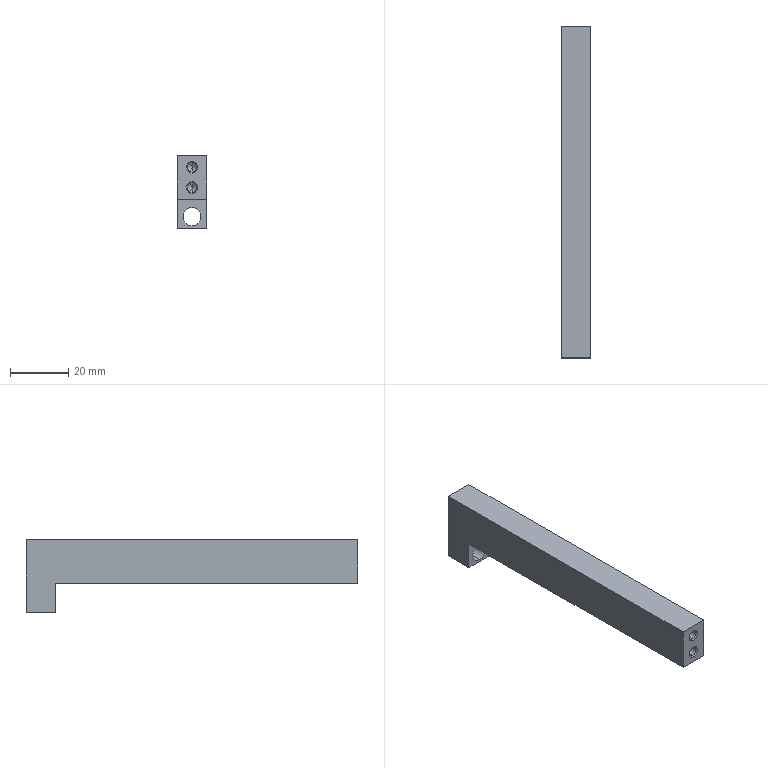Part | SolidWorks | features Extrusion 1, HoleWzd 1, ICE 1 | 1 solid | 22 faces | box 10 x 114 x 25 mm | volume 17594 mm3 | cone 8 | plane 8 | cylinder 6 | commonest cylinder face diameters 3.3 x4 6.2 x2
STEP:
#1=CARTESIAN_POINT('',(0.,0.375,-1.85));
#2=VERTEX_POINT('',#1);
#3=CARTESIAN_POINT('',(0.,0.375,-5.15));
#4=VERTEX_POINT('',#3);
#5=CARTESIAN_POINT('',(0.,0.375,-3.5));
#6=DIRECTION('',(0.,-1.,0.));
#7=DIRECTION('',(0.,0.,-1.));
#8=AXIS2_PLACEMENT_3D('',#5,#6,#7);
#9=CIRCLE('',#8,1.65);
#10=EDGE_CURVE('',#2,#4,#9,.T.);
#11=ORIENTED_EDGE('',*,*,#10,.F.);
#12=CARTESIAN_POINT('',(0.,0.,-1.475));
#13=VERTEX_POINT('',#12);
#14=CARTESIAN_POINT('',(0.,0.,-1.475));
#15=DIRECTION('',(0.,-0.7071,0.7071));
#16=VECTOR('',#15,1000.);
#17=LINE('',#14,#16);
#18=EDGE_CURVE('',#2,#13,#17,.T.);
#19=ORIENTED_EDGE('',*,*,#18,.T.);
#20=CARTESIAN_POINT('',(0.,0.,-5.525));
#21=VERTEX_POINT('',#20);
#22=CARTESIAN_POINT('',(0.,0.,-3.5));
#23=DIRECTION('',(0.,-1.,0.));
#24=DIRECTION('',(0.,0.,-1.));
#25=AXIS2_PLACEMENT_3D('',#22,#23,#24);
#26=CIRCLE('',#25,2.025);
#27=EDGE_CURVE('',#13,#21,#26,.T.);
#28=ORIENTED_EDGE('',*,*,#27,.T.);
#29=CARTESIAN_POINT('',(0.,0.,-5.525));
#30=DIRECTION('',(0.,-0.7071,-0.7071));
#31=VECTOR('',#30,1000.);
#32=LINE('',#29,#31);
#33=EDGE_CURVE('',#4,#21,#32,.T.);
#34=ORIENTED_EDGE('',*,*,#33,.F.);
#35=EDGE_LOOP('',(#11,#19,#28,#34));
#36=FACE_OUTER_BOUND('',#35,.T.);
#37=CARTESIAN_POINT('',(0.,0.,-3.5));
#38=DIRECTION('',(0.,-1.,0.));
#39=DIRECTION('',(0.,0.,-1.));
#40=AXIS2_PLACEMENT_3D('',#37,#38,#39);
#41=CONICAL_SURFACE('',#40,2.025,0.7854);
#42=ADVANCED_FACE('',(#36),#41,.F.);
#43=CARTESIAN_POINT('',(0.,11.5,-1.85));
#44=VERTEX_POINT('',#43);
#45=CARTESIAN_POINT('',(0.,11.5,-5.15));
#46=VERTEX_POINT('',#45);
#47=CARTESIAN_POINT('',(0.,11.5,-3.5));
#48=DIRECTION('',(0.,-1.,0.));
#49=DIRECTION('',(0.,0.,-1.));
#50=AXIS2_PLACEMENT_3D('',#47,#48,#49);
#51=CIRCLE('',#50,1.65);
#52=EDGE_CURVE('',#44,#46,#51,.T.);
#53=ORIENTED_EDGE('',*,*,#52,.F.);
#54=CARTESIAN_POINT('',(0.,0.,-1.85));
#55=DIRECTION('',(0.,-1.,0.));
#56=VECTOR('',#55,1000.);
#57=LINE('',#54,#56);
#58=EDGE_CURVE('',#44,#2,#57,.T.);
#59=ORIENTED_EDGE('',*,*,#58,.T.);
#60=ORIENTED_EDGE('',*,*,#10,.T.);
#61=CARTESIAN_POINT('',(0.,0.,-5.15));
#62=DIRECTION('',(0.,-1.,0.));
#63=VECTOR('',#62,1000.);
#64=LINE('',#61,#63);
#65=EDGE_CURVE('',#46,#4,#64,.T.);
#66=ORIENTED_EDGE('',*,*,#65,.F.);
#67=EDGE_LOOP('',(#53,#59,#60,#66));
#68=FACE_OUTER_BOUND('',#67,.T.);
#69=CARTESIAN_POINT('',(0.,0.,-3.5));
#70=DIRECTION('',(0.,-1.,0.));
#71=DIRECTION('',(0.,0.,-1.));
#72=AXIS2_PLACEMENT_3D('',#69,#70,#71);
#73=CYLINDRICAL_SURFACE('',#72,1.65);
#74=ADVANCED_FACE('',(#68),#73,.F.);
#75=CARTESIAN_POINT('',(0.,12.491,-3.5));
#76=VERTEX_POINT('',#75);
#77=CARTESIAN_POINT('',(0.,11.5,-5.15));
#78=DIRECTION('',(0.,-0.515,-0.8572));
#79=VECTOR('',#78,1000.);
#80=LINE('',#77,#79);
#81=EDGE_CURVE('',#76,#46,#80,.T.);
#82=ORIENTED_EDGE('',*,*,#81,.F.);
#83=CARTESIAN_POINT('',(0.,11.5,-1.85));
#84=DIRECTION('',(0.,-0.515,0.8572));
#85=VECTOR('',#84,1000.);
#86=LINE('',#83,#85);
#87=EDGE_CURVE('',#76,#44,#86,.T.);
#88=ORIENTED_EDGE('',*,*,#87,.T.);
#89=ORIENTED_EDGE('',*,*,#52,.T.);
#90=EDGE_LOOP('',(#82,#88,#89));
#91=FACE_OUTER_BOUND('',#90,.T.);
#92=CARTESIAN_POINT('',(0.,11.5,-3.5));
#93=DIRECTION('',(0.,-1.,0.));
#94=DIRECTION('',(0.,0.,-1.));
#95=AXIS2_PLACEMENT_3D('',#92,#93,#94);
#96=CONICAL_SURFACE('',#95,1.65,1.03);
#97=ADVANCED_FACE('',(#91),#96,.F.);
#98=CARTESIAN_POINT('',(0.,0.375,5.15));
#99=VERTEX_POINT('',#98);
#100=CARTESIAN_POINT('',(0.,0.375,1.85));
#101=VERTEX_POINT('',#100);
#102=CARTESIAN_POINT('',(0.,0.375,3.5));
#103=DIRECTION('',(0.,-1.,0.));
#104=DIRECTION('',(0.,0.,-1.));
#105=AXIS2_PLACEMENT_3D('',#102,#103,#104);
#106=CIRCLE('',#105,1.65);
#107=EDGE_CURVE('',#99,#101,#106,.T.);
#108=ORIENTED_EDGE('',*,*,#107,.F.);
#109=CARTESIAN_POINT('',(0.,0.,5.525));
#110=VERTEX_POINT('',#109);
#111=CARTESIAN_POINT('',(0.,0.,5.525));
#112=DIRECTION('',(0.,-0.7071,0.7071));
#113=VECTOR('',#112,1000.);
#114=LINE('',#111,#113);
#115=EDGE_CURVE('',#99,#110,#114,.T.);
#116=ORIENTED_EDGE('',*,*,#115,.T.);
#117=CARTESIAN_POINT('',(0.,0.,1.475));
#118=VERTEX_POINT('',#117);
#119=CARTESIAN_POINT('',(0.,0.,3.5));
#120=DIRECTION('',(0.,-1.,0.));
#121=DIRECTION('',(0.,0.,-1.));
#122=AXIS2_PLACEMENT_3D('',#119,#120,#121);
#123=CIRCLE('',#122,2.025);
#124=EDGE_CURVE('',#110,#118,#123,.T.);
#125=ORIENTED_EDGE('',*,*,#124,.T.);
#126=CARTESIAN_POINT('',(0.,0.,1.475));
#127=DIRECTION('',(0.,-0.7071,-0.7071));
#128=VECTOR('',#127,1000.);
#129=LINE('',#126,#128);
#130=EDGE_CURVE('',#101,#118,#129,.T.);
#131=ORIENTED_EDGE('',*,*,#130,.F.);
#132=EDGE_LOOP('',(#108,#116,#125,#131));
#133=FACE_OUTER_BOUND('',#132,.T.);
#134=CARTESIAN_POINT('',(0.,0.,3.5));
#135=DIRECTION('',(0.,-1.,0.));
#136=DIRECTION('',(0.,0.,-1.));
#137=AXIS2_PLACEMENT_3D('',#134,#135,#136);
#138=CONICAL_SURFACE('',#137,2.025,0.7854);
#139=ADVANCED_FACE('',(#133),#138,.F.);
#140=CARTESIAN_POINT('',(0.,11.5,5.15));
#141=VERTEX_POINT('',#140);
#142=CARTESIAN_POINT('',(0.,11.5,1.85));
#143=VERTEX_POINT('',#142);
#144=CARTESIAN_POINT('',(0.,11.5,3.5));
#145=DIRECTION('',(0.,-1.,0.));
#146=DIRECTION('',(0.,0.,-1.));
#147=AXIS2_PLACEMENT_3D('',#144,#145,#146);
#148=CIRCLE('',#147,1.65);
#149=EDGE_CURVE('',#141,#143,#148,.T.);
#150=ORIENTED_EDGE('',*,*,#149,.F.);
#151=CARTESIAN_POINT('',(0.,0.,5.15));
#152=DIRECTION('',(0.,-1.,0.));
#153=VECTOR('',#152,1000.);
#154=LINE('',#151,#153);
#155=EDGE_CURVE('',#141,#99,#154,.T.);
#156=ORIENTED_EDGE('',*,*,#155,.T.);
#157=ORIENTED_EDGE('',*,*,#107,.T.);
#158=CARTESIAN_POINT('',(0.,0.,1.85));
#159=DIRECTION('',(0.,-1.,0.));
#160=VECTOR('',#159,1000.);
#161=LINE('',#158,#160);
#162=EDGE_CURVE('',#143,#101,#161,.T.);
#163=ORIENTED_EDGE('',*,*,#162,.F.);
#164=EDGE_LOOP('',(#150,#156,#157,#163));
#165=FACE_OUTER_BOUND('',#164,.T.);
#166=CARTESIAN_POINT('',(0.,0.,3.5));
#167=DIRECTION('',(0.,-1.,0.));
#168=DIRECTION('',(0.,0.,-1.));
#169=AXIS2_PLACEMENT_3D('',#166,#167,#168);
#170=CYLINDRICAL_SURFACE('',#169,1.65);
#171=ADVANCED_FACE('',(#165),#170,.F.);
#172=CARTESIAN_POINT('',(0.,12.491,3.5));
#173=VERTEX_POINT('',#172);
#174=CARTESIAN_POINT('',(0.,11.5,1.85));
#175=DIRECTION('',(0.,-0.515,-0.8572));
#176=VECTOR('',#175,1000.);
#177=LINE('',#174,#176);
#178=EDGE_CURVE('',#173,#143,#177,.T.);
#179=ORIENTED_EDGE('',*,*,#178,.F.);
#180=CARTESIAN_POINT('',(0.,11.5,5.15));
#181=DIRECTION('',(0.,-0.515,0.8572));
#182=VECTOR('',#181,1000.);
#183=LINE('',#180,#182);
#184=EDGE_CURVE('',#173,#141,#183,.T.);
#185=ORIENTED_EDGE('',*,*,#184,.T.);
#186=ORIENTED_EDGE('',*,*,#149,.T.);
#187=EDGE_LOOP('',(#179,#185,#186));
#188=FACE_OUTER_BOUND('',#187,.T.);
#189=CARTESIAN_POINT('',(0.,11.5,3.5));
#190=DIRECTION('',(0.,-1.,0.));
#191=DIRECTION('',(0.,0.,-1.));
#192=AXIS2_PLACEMENT_3D('',#189,#190,#191);
#193=CONICAL_SURFACE('',#192,1.65,1.03);
#194=ADVANCED_FACE('',(#188),#193,.F.);
#195=CARTESIAN_POINT('',(0.,104.,-16.6));
#196=VERTEX_POINT('',#195);
#197=CARTESIAN_POINT('',(0.,104.,-10.4));
#198=VERTEX_POINT('',#197);
#199=CARTESIAN_POINT('',(0.,104.,-13.5));
#200=DIRECTION('',(0.,1.,0.));
#201=DIRECTION('',(0.,0.,1.));
#202=AXIS2_PLACEMENT_3D('',#199,#200,#201);
#203=CIRCLE('',#202,3.1);
#204=EDGE_CURVE('',#196,#198,#203,.T.);
#205=ORIENTED_EDGE('',*,*,#204,.F.);
#206=CARTESIAN_POINT('',(0.,114.,-16.6));
#207=VERTEX_POINT('',#206);
#208=CARTESIAN_POINT('',(0.,104.,-16.6));
#209=DIRECTION('',(0.,1.,0.));
#210=VECTOR('',#209,1000.);
#211=LINE('',#208,#210);
#212=EDGE_CURVE('',#196,#207,#211,.T.);
#213=ORIENTED_EDGE('',*,*,#212,.T.);
#214=CARTESIAN_POINT('',(0.,114.,-10.4));
#215=VERTEX_POINT('',#214);
#216=CARTESIAN_POINT('',(0.,114.,-13.5));
#217=DIRECTION('',(0.,1.,0.));
#218=DIRECTION('',(0.,0.,1.));
#219=AXIS2_PLACEMENT_3D('',#216,#217,#218);
#220=CIRCLE('',#219,3.1);
#221=EDGE_CURVE('',#207,#215,#220,.T.);
#222=ORIENTED_EDGE('',*,*,#221,.T.);
#223=CARTESIAN_POINT('',(0.,104.,-10.4));
#224=DIRECTION('',(0.,1.,0.));
#225=VECTOR('',#224,1000.);
#226=LINE('',#223,#225);
#227=EDGE_CURVE('',#198,#215,#226,.T.);
#228=ORIENTED_EDGE('',*,*,#227,.F.);
#229=EDGE_LOOP('',(#205,#213,#222,#228));
#230=FACE_OUTER_BOUND('',#229,.T.);
#231=CARTESIAN_POINT('',(0.,104.,-13.5));
#232=DIRECTION('',(0.,1.,0.));
#233=DIRECTION('',(0.,0.,1.));
#234=AXIS2_PLACEMENT_3D('',#231,#232,#233);
#235=CYLINDRICAL_SURFACE('',#234,3.1);
#236=ADVANCED_FACE('',(#230),#235,.F.);
#237=CARTESIAN_POINT('',(5.,0.,7.5));
#238=VERTEX_POINT('',#237);
#239=CARTESIAN_POINT('',(5.,0.,-7.5));
#240=VERTEX_POINT('',#239);
#241=CARTESIAN_POINT('',(5.,0.,7.5));
#242=DIRECTION('',(0.,0.,-1.));
#243=VECTOR('',#242,1000.);
#244=LINE('',#241,#243);
#245=EDGE_CURVE('',#238,#240,#244,.T.);
#246=ORIENTED_EDGE('',*,*,#245,.T.);
#247=CARTESIAN_POINT('',(5.,104.,-7.5));
#248=VERTEX_POINT('',#247);
#249=CARTESIAN_POINT('',(5.,114.,-7.5));
#250=DIRECTION('',(0.,-1.,0.));
#251=VECTOR('',#250,1000.);
#252=LINE('',#249,#251);
#253=EDGE_CURVE('',#248,#240,#252,.T.);
#254=ORIENTED_EDGE('',*,*,#253,.F.);
#255=CARTESIAN_POINT('',(5.,104.,-17.5));
#256=VERTEX_POINT('',#255);
#257=CARTESIAN_POINT('',(5.,104.,-7.5));
#258=DIRECTION('',(0.,0.,-1.));
#259=VECTOR('',#258,1000.);
#260=LINE('',#257,#259);
#261=EDGE_CURVE('',#248,#256,#260,.T.);
#262=ORIENTED_EDGE('',*,*,#261,.T.);
#263=CARTESIAN_POINT('',(5.,114.,-17.5));
#264=VERTEX_POINT('',#263);
#265=CARTESIAN_POINT('',(5.,104.,-17.5));
#266=DIRECTION('',(0.,1.,0.));
#267=VECTOR('',#266,1000.);
#268=LINE('',#265,#267);
#269=EDGE_CURVE('',#256,#264,#268,.T.);
#270=ORIENTED_EDGE('',*,*,#269,.T.);
#271=CARTESIAN_POINT('',(5.,114.,7.5));
#272=VERTEX_POINT('',#271);
#273=CARTESIAN_POINT('',(5.,114.,7.5));
#274=DIRECTION('',(0.,0.,-1.));
#275=VECTOR('',#274,1000.);
#276=LINE('',#273,#275);
#277=EDGE_CURVE('',#272,#264,#276,.T.);
#278=ORIENTED_EDGE('',*,*,#277,.F.);
#279=CARTESIAN_POINT('',(5.,114.,7.5));
#280=DIRECTION('',(0.,-1.,0.));
#281=VECTOR('',#280,1000.);
#282=LINE('',#279,#281);
#283=EDGE_CURVE('',#272,#238,#282,.T.);
#284=ORIENTED_EDGE('',*,*,#283,.T.);
#285=EDGE_LOOP('',(#246,#254,#262,#270,#278,#284));
#286=FACE_OUTER_BOUND('',#285,.T.);
#287=CARTESIAN_POINT('',(5.,114.,7.5));
#288=DIRECTION('',(-1.,0.,0.));
#289=DIRECTION('',(0.,0.,1.));
#290=AXIS2_PLACEMENT_3D('',#287,#288,#289);
#291=PLANE('',#290);
#292=ADVANCED_FACE('',(#286),#291,.F.);
#293=CARTESIAN_POINT('',(-5.,104.,-7.5));
#294=VERTEX_POINT('',#293);
#295=CARTESIAN_POINT('',(-5.,0.,-7.5));
#296=VERTEX_POINT('',#295);
#297=CARTESIAN_POINT('',(-5.,114.,-7.5));
#298=DIRECTION('',(0.,-1.,0.));
#299=VECTOR('',#298,1000.);
#300=LINE('',#297,#299);
#301=EDGE_CURVE('',#294,#296,#300,.T.);
#302=ORIENTED_EDGE('',*,*,#301,.F.);
#303=CARTESIAN_POINT('',(-5.,104.,-7.5));
#304=DIRECTION('',(1.,0.,0.));
#305=VECTOR('',#304,1000.);
#306=LINE('',#303,#305);
#307=EDGE_CURVE('',#294,#248,#306,.T.);
#308=ORIENTED_EDGE('',*,*,#307,.T.);
#309=ORIENTED_EDGE('',*,*,#253,.T.);
#310=CARTESIAN_POINT('',(-5.,0.,-7.5));
#311=DIRECTION('',(-1.,0.,0.));
#312=VECTOR('',#311,1000.);
#313=LINE('',#310,#312);
#314=EDGE_CURVE('',#240,#296,#313,.T.);
#315=ORIENTED_EDGE('',*,*,#314,.T.);
#316=EDGE_LOOP('',(#302,#308,#309,#315));
#317=FACE_OUTER_BOUND('',#316,.T.);
#318=CARTESIAN_POINT('',(-5.,114.,-7.5));
#319=DIRECTION('',(0.,0.,1.));
#320=DIRECTION('',(1.,0.,0.));
#321=AXIS2_PLACEMENT_3D('',#318,#319,#320);
#322=PLANE('',#321);
#323=ADVANCED_FACE('',(#317),#322,.F.);
#324=CARTESIAN_POINT('',(-5.,0.,7.5));
#325=VERTEX_POINT('',#324);
#326=CARTESIAN_POINT('',(-5.,0.,7.5));
#327=DIRECTION('',(0.,0.,1.));
#328=VECTOR('',#327,1000.);
#329=LINE('',#326,#328);
#330=EDGE_CURVE('',#296,#325,#329,.T.);
#331=ORIENTED_EDGE('',*,*,#330,.T.);
#332=CARTESIAN_POINT('',(-5.,114.,7.5));
#333=VERTEX_POINT('',#332);
#334=CARTESIAN_POINT('',(-5.,114.,7.5));
#335=DIRECTION('',(0.,-1.,0.));
#336=VECTOR('',#335,1000.);
#337=LINE('',#334,#336);
#338=EDGE_CURVE('',#333,#325,#337,.T.);
#339=ORIENTED_EDGE('',*,*,#338,.F.);
#340=CARTESIAN_POINT('',(-5.,114.,-17.5));
#341=VERTEX_POINT('',#340);
#342=CARTESIAN_POINT('',(-5.,114.,7.5));
#343=DIRECTION('',(0.,0.,1.));
#344=VECTOR('',#343,1000.);
#345=LINE('',#342,#344);
#346=EDGE_CURVE('',#341,#333,#345,.T.);
#347=ORIENTED_EDGE('',*,*,#346,.F.);
#348=CARTESIAN_POINT('',(-5.,104.,-17.5));
#349=VERTEX_POINT('',#348);
#350=CARTESIAN_POINT('',(-5.,104.,-17.5));
#351=DIRECTION('',(0.,1.,0.));
#352=VECTOR('',#351,1000.);
#353=LINE('',#350,#352);
#354=EDGE_CURVE('',#349,#341,#353,.T.);
#355=ORIENTED_EDGE('',*,*,#354,.F.);
#356=CARTESIAN_POINT('',(-5.,104.,-7.5));
#357=DIRECTION('',(0.,0.,1.));
#358=VECTOR('',#357,1000.);
#359=LINE('',#356,#358);
#360=EDGE_CURVE('',#349,#294,#359,.T.);
#361=ORIENTED_EDGE('',*,*,#360,.T.);
#362=ORIENTED_EDGE('',*,*,#301,.T.);
#363=EDGE_LOOP('',(#331,#339,#347,#355,#361,#362));
#364=FACE_OUTER_BOUND('',#363,.T.);
#365=CARTESIAN_POINT('',(-5.,114.,7.5));
#366=DIRECTION('',(1.,0.,0.));
#367=DIRECTION('',(0.,0.,-1.));
#368=AXIS2_PLACEMENT_3D('',#365,#366,#367);
#369=PLANE('',#368);
#370=ADVANCED_FACE('',(#364),#369,.F.);
#371=CARTESIAN_POINT('',(-5.,0.,7.5));
#372=DIRECTION('',(1.,0.,0.));
#373=VECTOR('',#372,1000.);
#374=LINE('',#371,#373);
#375=EDGE_CURVE('',#325,#238,#374,.T.);
#376=ORIENTED_EDGE('',*,*,#375,.T.);
#377=ORIENTED_EDGE('',*,*,#283,.F.);
#378=CARTESIAN_POINT('',(-5.,114.,7.5));
#379=DIRECTION('',(1.,0.,0.));
#380=VECTOR('',#379,1000.);
#381=LINE('',#378,#380);
#382=EDGE_CURVE('',#333,#272,#381,.T.);
#383=ORIENTED_EDGE('',*,*,#382,.F.);
#384=ORIENTED_EDGE('',*,*,#338,.T.);
#385=EDGE_LOOP('',(#376,#377,#383,#384));
#386=FACE_OUTER_BOUND('',#385,.T.);
#387=CARTESIAN_POINT('',(-5.,114.,7.5));
#388=DIRECTION('',(0.,0.,-1.));
#389=DIRECTION('',(-1.,0.,0.));
#390=AXIS2_PLACEMENT_3D('',#387,#388,#389);
#391=PLANE('',#390);
#392=ADVANCED_FACE('',(#386),#391,.F.);
#393=ORIENTED_EDGE('',*,*,#277,.T.);
#394=CARTESIAN_POINT('',(-5.,114.,-17.5));
#395=DIRECTION('',(-1.,0.,0.));
#396=VECTOR('',#395,1000.);
#397=LINE('',#394,#396);
#398=EDGE_CURVE('',#264,#341,#397,.T.);
#399=ORIENTED_EDGE('',*,*,#398,.T.);
#400=ORIENTED_EDGE('',*,*,#346,.T.);
#401=ORIENTED_EDGE('',*,*,#382,.T.);
#402=EDGE_LOOP('',(#393,#399,#400,#401));
#403=FACE_OUTER_BOUND('',#402,.T.);
#404=CARTESIAN_POINT('',(0.,114.,-13.5));
#405=DIRECTION('',(0.,1.,0.));
#406=DIRECTION('',(0.,0.,1.));
#407=AXIS2_PLACEMENT_3D('',#404,#405,#406);
#408=CIRCLE('',#407,3.1);
#409=EDGE_CURVE('',#215,#207,#408,.T.);
#410=ORIENTED_EDGE('',*,*,#409,.F.);
#411=ORIENTED_EDGE('',*,*,#221,.F.);
#412=EDGE_LOOP('',(#410,#411));
#413=FACE_BOUND('',#412,.T.);
#414=CARTESIAN_POINT('',(0.,114.,0.));
#415=DIRECTION('',(0.,-1.,0.));
#416=DIRECTION('',(0.,0.,-1.));
#417=AXIS2_PLACEMENT_3D('',#414,#415,#416);
#418=PLANE('',#417);
#419=ADVANCED_FACE('',(#403,#413),#418,.F.);
#420=CARTESIAN_POINT('',(0.,0.,-3.5));
#421=DIRECTION('',(0.,-1.,0.));
#422=DIRECTION('',(0.,0.,-1.));
#423=AXIS2_PLACEMENT_3D('',#420,#421,#422);
#424=CIRCLE('',#423,2.025);
#425=EDGE_CURVE('',#21,#13,#424,.T.);
#426=ORIENTED_EDGE('',*,*,#425,.F.);
#427=ORIENTED_EDGE('',*,*,#27,.F.);
#428=EDGE_LOOP('',(#426,#427));
#429=FACE_BOUND('',#428,.T.);
#430=CARTESIAN_POINT('',(0.,0.,3.5));
#431=DIRECTION('',(0.,-1.,0.));
#432=DIRECTION('',(0.,0.,-1.));
#433=AXIS2_PLACEMENT_3D('',#430,#431,#432);
#434=CIRCLE('',#433,2.025);
#435=EDGE_CURVE('',#118,#110,#434,.T.);
#436=ORIENTED_EDGE('',*,*,#435,.F.);
#437=ORIENTED_EDGE('',*,*,#124,.F.);
#438=EDGE_LOOP('',(#436,#437));
#439=FACE_BOUND('',#438,.T.);
#440=ORIENTED_EDGE('',*,*,#245,.F.);
#441=ORIENTED_EDGE('',*,*,#375,.F.);
#442=ORIENTED_EDGE('',*,*,#330,.F.);
#443=ORIENTED_EDGE('',*,*,#314,.F.);
#444=EDGE_LOOP('',(#440,#441,#442,#443));
#445=FACE_OUTER_BOUND('',#444,.T.);
#446=CARTESIAN_POINT('',(0.,0.,0.));
#447=DIRECTION('',(0.,-1.,0.));
#448=DIRECTION('',(0.,0.,-1.));
#449=AXIS2_PLACEMENT_3D('',#446,#447,#448);
#450=PLANE('',#449);
#451=ADVANCED_FACE('',(#429,#439,#445),#450,.T.);
#452=ORIENTED_EDGE('',*,*,#398,.F.);
#453=ORIENTED_EDGE('',*,*,#269,.F.);
#454=CARTESIAN_POINT('',(-5.,104.,-17.5));
#455=DIRECTION('',(-1.,0.,0.));
#456=VECTOR('',#455,1000.);
#457=LINE('',#454,#456);
#458=EDGE_CURVE('',#256,#349,#457,.T.);
#459=ORIENTED_EDGE('',*,*,#458,.T.);
#460=ORIENTED_EDGE('',*,*,#354,.T.);
#461=EDGE_LOOP('',(#452,#453,#459,#460));
#462=FACE_OUTER_BOUND('',#461,.T.);
#463=CARTESIAN_POINT('',(-5.,104.,-17.5));
#464=DIRECTION('',(0.,0.,-1.));
#465=DIRECTION('',(-1.,0.,0.));
#466=AXIS2_PLACEMENT_3D('',#463,#464,#465);
#467=PLANE('',#466);
#468=ADVANCED_FACE('',(#462),#467,.T.);
#469=CARTESIAN_POINT('',(0.,104.,-13.5));
#470=DIRECTION('',(0.,1.,0.));
#471=DIRECTION('',(0.,0.,1.));
#472=AXIS2_PLACEMENT_3D('',#469,#470,#471);
#473=CIRCLE('',#472,3.1);
#474=EDGE_CURVE('',#198,#196,#473,.T.);
#475=ORIENTED_EDGE('',*,*,#474,.T.);
#476=ORIENTED_EDGE('',*,*,#204,.T.);
#477=EDGE_LOOP('',(#475,#476));
#478=FACE_BOUND('',#477,.T.);
#479=ORIENTED_EDGE('',*,*,#360,.F.);
#480=ORIENTED_EDGE('',*,*,#458,.F.);
#481=ORIENTED_EDGE('',*,*,#261,.F.);
#482=ORIENTED_EDGE('',*,*,#307,.F.);
#483=EDGE_LOOP('',(#479,#480,#481,#482));
#484=FACE_OUTER_BOUND('',#483,.T.);
#485=CARTESIAN_POINT('',(0.,104.,0.));
#486=DIRECTION('',(0.,-1.,0.));
#487=DIRECTION('',(0.,0.,-1.));
#488=AXIS2_PLACEMENT_3D('',#485,#486,#487);
#489=PLANE('',#488);
#490=ADVANCED_FACE('',(#478,#484),#489,.T.);
#491=ORIENTED_EDGE('',*,*,#212,.F.);
#492=ORIENTED_EDGE('',*,*,#474,.F.);
#493=ORIENTED_EDGE('',*,*,#227,.T.);
#494=ORIENTED_EDGE('',*,*,#409,.T.);
#495=EDGE_LOOP('',(#491,#492,#493,#494));
#496=FACE_OUTER_BOUND('',#495,.T.);
#497=CARTESIAN_POINT('',(0.,104.,-13.5));
#498=DIRECTION('',(0.,1.,0.));
#499=DIRECTION('',(0.,0.,1.));
#500=AXIS2_PLACEMENT_3D('',#497,#498,#499);
#501=CYLINDRICAL_SURFACE('',#500,3.1);
#502=ADVANCED_FACE('',(#496),#501,.F.);
#503=ORIENTED_EDGE('',*,*,#184,.F.);
#504=ORIENTED_EDGE('',*,*,#178,.T.);
#505=CARTESIAN_POINT('',(0.,11.5,3.5));
#506=DIRECTION('',(0.,-1.,0.));
#507=DIRECTION('',(0.,0.,-1.));
#508=AXIS2_PLACEMENT_3D('',#505,#506,#507);
#509=CIRCLE('',#508,1.65);
#510=EDGE_CURVE('',#143,#141,#509,.T.);
#511=ORIENTED_EDGE('',*,*,#510,.T.);
#512=EDGE_LOOP('',(#503,#504,#511));
#513=FACE_OUTER_BOUND('',#512,.T.);
#514=CARTESIAN_POINT('',(0.,11.5,3.5));
#515=DIRECTION('',(0.,-1.,0.));
#516=DIRECTION('',(0.,0.,-1.));
#517=AXIS2_PLACEMENT_3D('',#514,#515,#516);
#518=CONICAL_SURFACE('',#517,1.65,1.03);
#519=ADVANCED_FACE('',(#513),#518,.F.);
#520=ORIENTED_EDGE('',*,*,#155,.F.);
#521=ORIENTED_EDGE('',*,*,#510,.F.);
#522=ORIENTED_EDGE('',*,*,#162,.T.);
#523=CARTESIAN_POINT('',(0.,0.375,3.5));
#524=DIRECTION('',(0.,-1.,0.));
#525=DIRECTION('',(0.,0.,-1.));
#526=AXIS2_PLACEMENT_3D('',#523,#524,#525);
#527=CIRCLE('',#526,1.65);
#528=EDGE_CURVE('',#101,#99,#527,.T.);
#529=ORIENTED_EDGE('',*,*,#528,.T.);
#530=EDGE_LOOP('',(#520,#521,#522,#529));
#531=FACE_OUTER_BOUND('',#530,.T.);
#532=CARTESIAN_POINT('',(0.,0.,3.5));
#533=DIRECTION('',(0.,-1.,0.));
#534=DIRECTION('',(0.,0.,-1.));
#535=AXIS2_PLACEMENT_3D('',#532,#533,#534);
#536=CYLINDRICAL_SURFACE('',#535,1.65);
#537=ADVANCED_FACE('',(#531),#536,.F.);
#538=ORIENTED_EDGE('',*,*,#115,.F.);
#539=ORIENTED_EDGE('',*,*,#528,.F.);
#540=ORIENTED_EDGE('',*,*,#130,.T.);
#541=ORIENTED_EDGE('',*,*,#435,.T.);
#542=EDGE_LOOP('',(#538,#539,#540,#541));
#543=FACE_OUTER_BOUND('',#542,.T.);
#544=CARTESIAN_POINT('',(0.,0.,3.5));
#545=DIRECTION('',(0.,-1.,0.));
#546=DIRECTION('',(0.,0.,-1.));
#547=AXIS2_PLACEMENT_3D('',#544,#545,#546);
#548=CONICAL_SURFACE('',#547,2.025,0.7854);
#549=ADVANCED_FACE('',(#543),#548,.F.);
#550=ORIENTED_EDGE('',*,*,#87,.F.);
#551=ORIENTED_EDGE('',*,*,#81,.T.);
#552=CARTESIAN_POINT('',(0.,11.5,-3.5));
#553=DIRECTION('',(0.,-1.,0.));
#554=DIRECTION('',(0.,0.,-1.));
#555=AXIS2_PLACEMENT_3D('',#552,#553,#554);
#556=CIRCLE('',#555,1.65);
#557=EDGE_CURVE('',#46,#44,#556,.T.);
#558=ORIENTED_EDGE('',*,*,#557,.T.);
#559=EDGE_LOOP('',(#550,#551,#558));
#560=FACE_OUTER_BOUND('',#559,.T.);
#561=CARTESIAN_POINT('',(0.,11.5,-3.5));
#562=DIRECTION('',(0.,-1.,0.));
#563=DIRECTION('',(0.,0.,-1.));
#564=AXIS2_PLACEMENT_3D('',#561,#562,#563);
#565=CONICAL_SURFACE('',#564,1.65,1.03);
#566=ADVANCED_FACE('',(#560),#565,.F.);
#567=ORIENTED_EDGE('',*,*,#58,.F.);
#568=ORIENTED_EDGE('',*,*,#557,.F.);
#569=ORIENTED_EDGE('',*,*,#65,.T.);
#570=CARTESIAN_POINT('',(0.,0.375,-3.5));
#571=DIRECTION('',(0.,-1.,0.));
#572=DIRECTION('',(0.,0.,-1.));
#573=AXIS2_PLACEMENT_3D('',#570,#571,#572);
#574=CIRCLE('',#573,1.65);
#575=EDGE_CURVE('',#4,#2,#574,.T.);
#576=ORIENTED_EDGE('',*,*,#575,.T.);
#577=EDGE_LOOP('',(#567,#568,#569,#576));
#578=FACE_OUTER_BOUND('',#577,.T.);
#579=CARTESIAN_POINT('',(0.,0.,-3.5));
#580=DIRECTION('',(0.,-1.,0.));
#581=DIRECTION('',(0.,0.,-1.));
#582=AXIS2_PLACEMENT_3D('',#579,#580,#581);
#583=CYLINDRICAL_SURFACE('',#582,1.65);
#584=ADVANCED_FACE('',(#578),#583,.F.);
#585=ORIENTED_EDGE('',*,*,#18,.F.);
#586=ORIENTED_EDGE('',*,*,#575,.F.);
#587=ORIENTED_EDGE('',*,*,#33,.T.);
#588=ORIENTED_EDGE('',*,*,#425,.T.);
#589=EDGE_LOOP('',(#585,#586,#587,#588));
#590=FACE_OUTER_BOUND('',#589,.T.);
#591=CARTESIAN_POINT('',(0.,0.,-3.5));
#592=DIRECTION('',(0.,-1.,0.));
#593=DIRECTION('',(0.,0.,-1.));
#594=AXIS2_PLACEMENT_3D('',#591,#592,#593);
#595=CONICAL_SURFACE('',#594,2.025,0.7854);
#596=ADVANCED_FACE('',(#590),#595,.F.);
#597=CLOSED_SHELL('',(#42,#74,#97,#139,#171,#194,#236,#292,#323,#370,#392,#419,#451,#468,#490,#502,#519,#537,#549,#566,#584,#596));
#598=MANIFOLD_SOLID_BREP('',#597);
#599=CARTESIAN_POINT('',(0.,0.,0.));
#600=DIRECTION('',(0.,0.,1.));
#601=DIRECTION('',(1.,0.,0.));
#602=AXIS2_PLACEMENT_3D('',#599,#600,#601);
#603=(LENGTH_UNIT()NAMED_UNIT(*)SI_UNIT(.MILLI.,.METRE.));
#604=UNCERTAINTY_MEASURE_WITH_UNIT(LENGTH_MEASURE(0.00001),#603,'','');
#605=(NAMED_UNIT(*)PLANE_ANGLE_UNIT()SI_UNIT($,.RADIAN.));
#606=(NAMED_UNIT(*)SI_UNIT($,.STERADIAN.)SOLID_ANGLE_UNIT());
#607=(GEOMETRIC_REPRESENTATION_CONTEXT(3)GLOBAL_UNCERTAINTY_ASSIGNED_CONTEXT((#604))GLOBAL_UNIT_ASSIGNED_CONTEXT((#603,#605,#606))REPRESENTATION_CONTEXT('',''));
#608=ADVANCED_BREP_SHAPE_REPRESENTATION('',(#598,#602),#607);